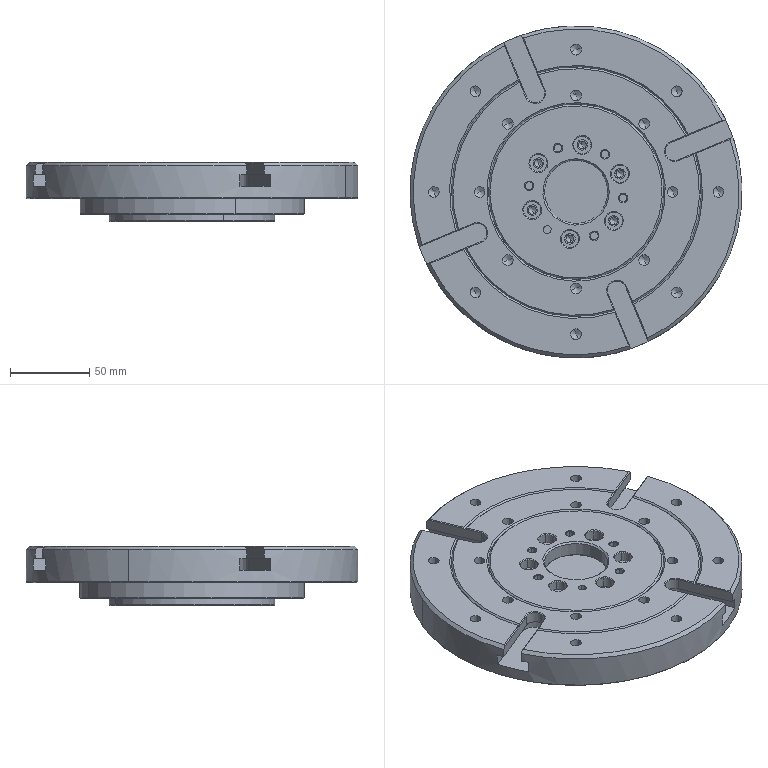Part | 2 solids | 367 faces | volume 799439 mm3 | cylinder 164 | cone 118 | plane 85 | commonest cylinder face diameters 6.6 x36 11 x36 6.8 x32 5 x24 12 x4 21 x4